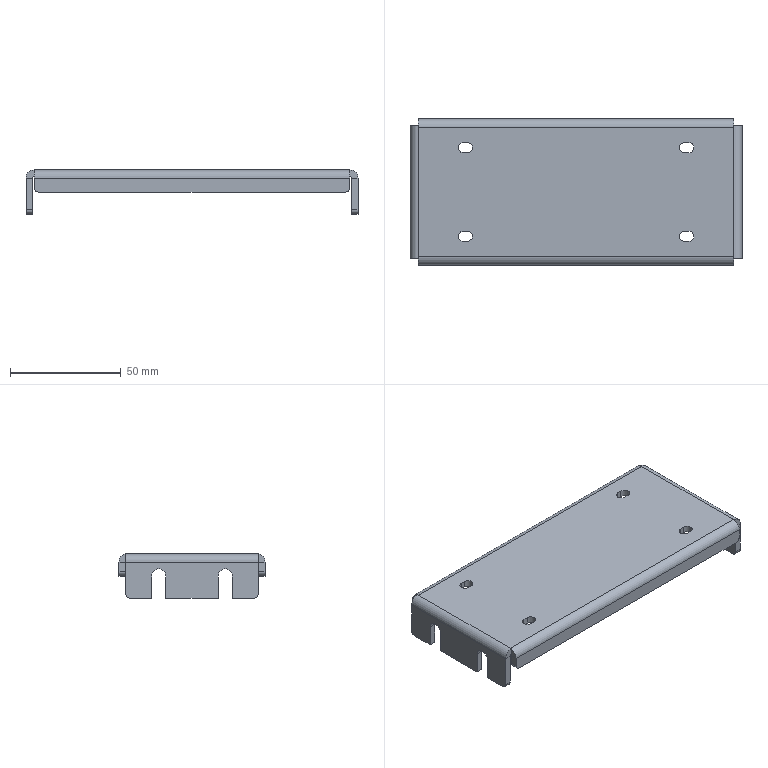Part | STEP file | 04-24 guide post fixing plate (Default) | 1 solid | 88 faces | box 150 x 66 x 20 mm | volume 39207 mm3 | plane 54 | cylinder 34 | commonest cylinder face diameters 4.5 x12 4 x8 6.5 x6 1.473 x4 7.473 x4